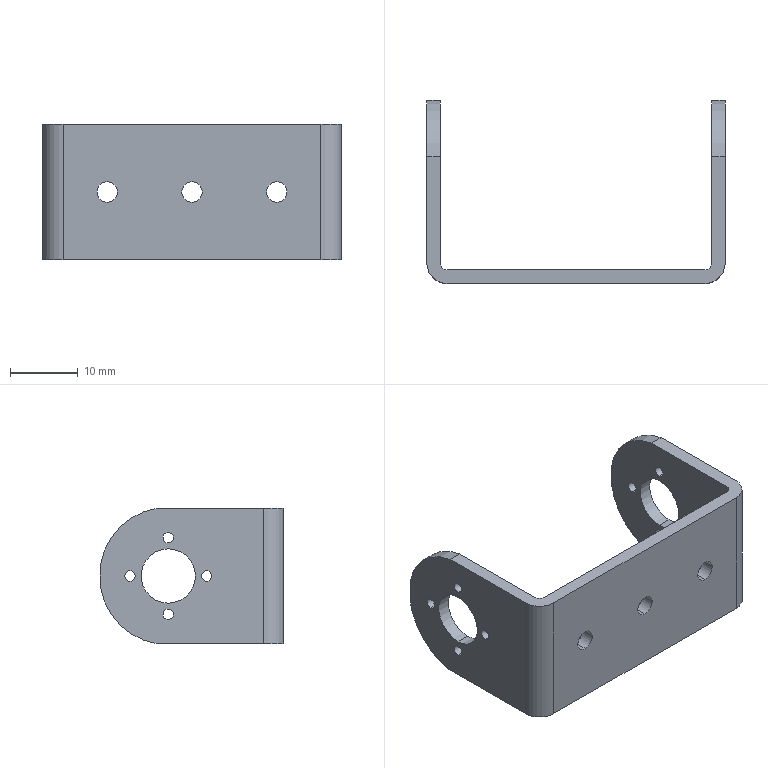Part | SolidWorks | features ICE 2, Extrusion 1 | 1 solid | 44 faces | box 44 x 27 x 20 mm | volume 3261 mm3 | cylinder 34 | plane 10 | commonest cylinder face diameters 1.543 x16 3 x6 8 x4 20.27 x4 2 x2 6 x2
STEP:
#1=CARTESIAN_POINT('',(7.5,-2.,8.5));
#2=VERTEX_POINT('',#1);
#3=CARTESIAN_POINT('',(7.5,-2.,11.5));
#4=VERTEX_POINT('',#3);
#5=CARTESIAN_POINT('',(7.5,-2.,10.));
#6=DIRECTION('',(0.,1.,0.));
#7=DIRECTION('',(0.,0.,1.));
#8=AXIS2_PLACEMENT_3D('',#5,#6,#7);
#9=CIRCLE('',#8,1.5);
#10=EDGE_CURVE('',#2,#4,#9,.T.);
#11=ORIENTED_EDGE('',*,*,#10,.F.);
#12=CARTESIAN_POINT('',(7.5,0.,8.5));
#13=VERTEX_POINT('',#12);
#14=CARTESIAN_POINT('',(7.5,-2.,8.5));
#15=DIRECTION('',(0.,1.,0.));
#16=VECTOR('',#15,1000.);
#17=LINE('',#14,#16);
#18=EDGE_CURVE('',#2,#13,#17,.T.);
#19=ORIENTED_EDGE('',*,*,#18,.T.);
#20=CARTESIAN_POINT('',(7.5,0.,11.5));
#21=VERTEX_POINT('',#20);
#22=CARTESIAN_POINT('',(7.5,0.,10.));
#23=DIRECTION('',(0.,1.,0.));
#24=DIRECTION('',(0.,0.,1.));
#25=AXIS2_PLACEMENT_3D('',#22,#23,#24);
#26=CIRCLE('',#25,1.5);
#27=EDGE_CURVE('',#13,#21,#26,.T.);
#28=ORIENTED_EDGE('',*,*,#27,.T.);
#29=CARTESIAN_POINT('',(7.5,-2.,11.5));
#30=DIRECTION('',(0.,1.,0.));
#31=VECTOR('',#30,1000.);
#32=LINE('',#29,#31);
#33=EDGE_CURVE('',#4,#21,#32,.T.);
#34=ORIENTED_EDGE('',*,*,#33,.F.);
#35=EDGE_LOOP('',(#11,#19,#28,#34));
#36=FACE_OUTER_BOUND('',#35,.T.);
#37=CARTESIAN_POINT('',(7.5,-2.,10.));
#38=DIRECTION('',(0.,1.,0.));
#39=DIRECTION('',(0.,0.,1.));
#40=AXIS2_PLACEMENT_3D('',#37,#38,#39);
#41=CYLINDRICAL_SURFACE('',#40,1.5);
#42=ADVANCED_FACE('',(#36),#41,.F.);
#43=CARTESIAN_POINT('',(20.,-2.,8.5));
#44=VERTEX_POINT('',#43);
#45=CARTESIAN_POINT('',(20.,-2.,11.5));
#46=VERTEX_POINT('',#45);
#47=CARTESIAN_POINT('',(20.,-2.,10.));
#48=DIRECTION('',(0.,1.,0.));
#49=DIRECTION('',(0.,0.,1.));
#50=AXIS2_PLACEMENT_3D('',#47,#48,#49);
#51=CIRCLE('',#50,1.5);
#52=EDGE_CURVE('',#44,#46,#51,.T.);
#53=ORIENTED_EDGE('',*,*,#52,.F.);
#54=CARTESIAN_POINT('',(20.,0.,8.5));
#55=VERTEX_POINT('',#54);
#56=CARTESIAN_POINT('',(20.,-2.,8.5));
#57=DIRECTION('',(0.,1.,0.));
#58=VECTOR('',#57,1000.);
#59=LINE('',#56,#58);
#60=EDGE_CURVE('',#44,#55,#59,.T.);
#61=ORIENTED_EDGE('',*,*,#60,.T.);
#62=CARTESIAN_POINT('',(20.,0.,11.5));
#63=VERTEX_POINT('',#62);
#64=CARTESIAN_POINT('',(20.,0.,10.));
#65=DIRECTION('',(0.,1.,0.));
#66=DIRECTION('',(0.,0.,1.));
#67=AXIS2_PLACEMENT_3D('',#64,#65,#66);
#68=CIRCLE('',#67,1.5);
#69=EDGE_CURVE('',#55,#63,#68,.T.);
#70=ORIENTED_EDGE('',*,*,#69,.T.);
#71=CARTESIAN_POINT('',(20.,-2.,11.5));
#72=DIRECTION('',(0.,1.,0.));
#73=VECTOR('',#72,1000.);
#74=LINE('',#71,#73);
#75=EDGE_CURVE('',#46,#63,#74,.T.);
#76=ORIENTED_EDGE('',*,*,#75,.F.);
#77=EDGE_LOOP('',(#53,#61,#70,#76));
#78=FACE_OUTER_BOUND('',#77,.T.);
#79=CARTESIAN_POINT('',(20.,-2.,10.));
#80=DIRECTION('',(0.,1.,0.));
#81=DIRECTION('',(0.,0.,1.));
#82=AXIS2_PLACEMENT_3D('',#79,#80,#81);
#83=CYLINDRICAL_SURFACE('',#82,1.5);
#84=ADVANCED_FACE('',(#78),#83,.F.);
#85=CARTESIAN_POINT('',(32.5,-2.,8.5));
#86=VERTEX_POINT('',#85);
#87=CARTESIAN_POINT('',(32.5,-2.,11.5));
#88=VERTEX_POINT('',#87);
#89=CARTESIAN_POINT('',(32.5,-2.,10.));
#90=DIRECTION('',(0.,1.,0.));
#91=DIRECTION('',(0.,0.,1.));
#92=AXIS2_PLACEMENT_3D('',#89,#90,#91);
#93=CIRCLE('',#92,1.5);
#94=EDGE_CURVE('',#86,#88,#93,.T.);
#95=ORIENTED_EDGE('',*,*,#94,.F.);
#96=CARTESIAN_POINT('',(32.5,0.,8.5));
#97=VERTEX_POINT('',#96);
#98=CARTESIAN_POINT('',(32.5,-2.,8.5));
#99=DIRECTION('',(0.,1.,0.));
#100=VECTOR('',#99,1000.);
#101=LINE('',#98,#100);
#102=EDGE_CURVE('',#86,#97,#101,.T.);
#103=ORIENTED_EDGE('',*,*,#102,.T.);
#104=CARTESIAN_POINT('',(32.5,0.,11.5));
#105=VERTEX_POINT('',#104);
#106=CARTESIAN_POINT('',(32.5,0.,10.));
#107=DIRECTION('',(0.,1.,0.));
#108=DIRECTION('',(0.,0.,1.));
#109=AXIS2_PLACEMENT_3D('',#106,#107,#108);
#110=CIRCLE('',#109,1.5);
#111=EDGE_CURVE('',#97,#105,#110,.T.);
#112=ORIENTED_EDGE('',*,*,#111,.T.);
#113=CARTESIAN_POINT('',(32.5,-2.,11.5));
#114=DIRECTION('',(0.,1.,0.));
#115=VECTOR('',#114,1000.);
#116=LINE('',#113,#115);
#117=EDGE_CURVE('',#88,#105,#116,.T.);
#118=ORIENTED_EDGE('',*,*,#117,.F.);
#119=EDGE_LOOP('',(#95,#103,#112,#118));
#120=FACE_OUTER_BOUND('',#119,.T.);
#121=CARTESIAN_POINT('',(32.5,-2.,10.));
#122=DIRECTION('',(0.,1.,0.));
#123=DIRECTION('',(0.,0.,1.));
#124=AXIS2_PLACEMENT_3D('',#121,#122,#123);
#125=CYLINDRICAL_SURFACE('',#124,1.5);
#126=ADVANCED_FACE('',(#120),#125,.F.);
#127=CARTESIAN_POINT('',(42.,9.349,9.229));
#128=VERTEX_POINT('',#127);
#129=CARTESIAN_POINT('',(42.,9.349,10.771));
#130=VERTEX_POINT('',#129);
#131=CARTESIAN_POINT('',(42.,9.349,10.));
#132=DIRECTION('',(-1.,0.,0.));
#133=DIRECTION('',(0.,0.,1.));
#134=AXIS2_PLACEMENT_3D('',#131,#132,#133);
#135=CIRCLE('',#134,0.7713);
#136=EDGE_CURVE('',#128,#130,#135,.T.);
#137=ORIENTED_EDGE('',*,*,#136,.F.);
#138=CARTESIAN_POINT('',(40.,9.349,9.229));
#139=VERTEX_POINT('',#138);
#140=CARTESIAN_POINT('',(42.,9.349,9.229));
#141=DIRECTION('',(-1.,0.,0.));
#142=VECTOR('',#141,1000.);
#143=LINE('',#140,#142);
#144=EDGE_CURVE('',#128,#139,#143,.T.);
#145=ORIENTED_EDGE('',*,*,#144,.T.);
#146=CARTESIAN_POINT('',(40.,9.349,10.771));
#147=VERTEX_POINT('',#146);
#148=CARTESIAN_POINT('',(40.,9.349,10.));
#149=DIRECTION('',(1.,0.,0.));
#150=DIRECTION('',(0.,0.,-1.));
#151=AXIS2_PLACEMENT_3D('',#148,#149,#150);
#152=CIRCLE('',#151,0.7713);
#153=EDGE_CURVE('',#147,#139,#152,.T.);
#154=ORIENTED_EDGE('',*,*,#153,.F.);
#155=CARTESIAN_POINT('',(42.,9.349,10.771));
#156=DIRECTION('',(-1.,0.,0.));
#157=VECTOR('',#156,1000.);
#158=LINE('',#155,#157);
#159=EDGE_CURVE('',#130,#147,#158,.T.);
#160=ORIENTED_EDGE('',*,*,#159,.F.);
#161=EDGE_LOOP('',(#137,#145,#154,#160));
#162=FACE_OUTER_BOUND('',#161,.T.);
#163=CARTESIAN_POINT('',(42.,9.349,10.));
#164=DIRECTION('',(-1.,0.,0.));
#165=DIRECTION('',(0.,0.,1.));
#166=AXIS2_PLACEMENT_3D('',#163,#164,#165);
#167=CYLINDRICAL_SURFACE('',#166,0.7713);
#168=ADVANCED_FACE('',(#162),#167,.F.);
#169=CARTESIAN_POINT('',(42.,15.,14.88));
#170=VERTEX_POINT('',#169);
#171=CARTESIAN_POINT('',(42.,15.,16.423));
#172=VERTEX_POINT('',#171);
#173=CARTESIAN_POINT('',(42.,15.,15.651));
#174=DIRECTION('',(-1.,0.,0.));
#175=DIRECTION('',(0.,0.,1.));
#176=AXIS2_PLACEMENT_3D('',#173,#174,#175);
#177=CIRCLE('',#176,0.7713);
#178=EDGE_CURVE('',#170,#172,#177,.T.);
#179=ORIENTED_EDGE('',*,*,#178,.F.);
#180=CARTESIAN_POINT('',(40.,15.,14.88));
#181=VERTEX_POINT('',#180);
#182=CARTESIAN_POINT('',(42.,15.,14.88));
#183=DIRECTION('',(-1.,0.,0.));
#184=VECTOR('',#183,1000.);
#185=LINE('',#182,#184);
#186=EDGE_CURVE('',#170,#181,#185,.T.);
#187=ORIENTED_EDGE('',*,*,#186,.T.);
#188=CARTESIAN_POINT('',(40.,15.,16.423));
#189=VERTEX_POINT('',#188);
#190=CARTESIAN_POINT('',(40.,15.,15.651));
#191=DIRECTION('',(1.,0.,0.));
#192=DIRECTION('',(0.,0.,-1.));
#193=AXIS2_PLACEMENT_3D('',#190,#191,#192);
#194=CIRCLE('',#193,0.7713);
#195=EDGE_CURVE('',#189,#181,#194,.T.);
#196=ORIENTED_EDGE('',*,*,#195,.F.);
#197=CARTESIAN_POINT('',(42.,15.,16.423));
#198=DIRECTION('',(-1.,0.,0.));
#199=VECTOR('',#198,1000.);
#200=LINE('',#197,#199);
#201=EDGE_CURVE('',#172,#189,#200,.T.);
#202=ORIENTED_EDGE('',*,*,#201,.F.);
#203=EDGE_LOOP('',(#179,#187,#196,#202));
#204=FACE_OUTER_BOUND('',#203,.T.);
#205=CARTESIAN_POINT('',(42.,15.,15.651));
#206=DIRECTION('',(-1.,0.,0.));
#207=DIRECTION('',(0.,0.,1.));
#208=AXIS2_PLACEMENT_3D('',#205,#206,#207);
#209=CYLINDRICAL_SURFACE('',#208,0.7713);
#210=ADVANCED_FACE('',(#204),#209,.F.);
#211=CARTESIAN_POINT('',(42.,20.651,9.229));
#212=VERTEX_POINT('',#211);
#213=CARTESIAN_POINT('',(42.,20.651,10.771));
#214=VERTEX_POINT('',#213);
#215=CARTESIAN_POINT('',(42.,20.651,10.));
#216=DIRECTION('',(-1.,0.,0.));
#217=DIRECTION('',(0.,0.,1.));
#218=AXIS2_PLACEMENT_3D('',#215,#216,#217);
#219=CIRCLE('',#218,0.7713);
#220=EDGE_CURVE('',#212,#214,#219,.T.);
#221=ORIENTED_EDGE('',*,*,#220,.F.);
#222=CARTESIAN_POINT('',(40.,20.651,9.229));
#223=VERTEX_POINT('',#222);
#224=CARTESIAN_POINT('',(42.,20.651,9.229));
#225=DIRECTION('',(-1.,0.,0.));
#226=VECTOR('',#225,1000.);
#227=LINE('',#224,#226);
#228=EDGE_CURVE('',#212,#223,#227,.T.);
#229=ORIENTED_EDGE('',*,*,#228,.T.);
#230=CARTESIAN_POINT('',(40.,20.651,10.771));
#231=VERTEX_POINT('',#230);
#232=CARTESIAN_POINT('',(40.,20.651,10.));
#233=DIRECTION('',(1.,0.,0.));
#234=DIRECTION('',(0.,0.,-1.));
#235=AXIS2_PLACEMENT_3D('',#232,#233,#234);
#236=CIRCLE('',#235,0.7713);
#237=EDGE_CURVE('',#231,#223,#236,.T.);
#238=ORIENTED_EDGE('',*,*,#237,.F.);
#239=CARTESIAN_POINT('',(42.,20.651,10.771));
#240=DIRECTION('',(-1.,0.,0.));
#241=VECTOR('',#240,1000.);
#242=LINE('',#239,#241);
#243=EDGE_CURVE('',#214,#231,#242,.T.);
#244=ORIENTED_EDGE('',*,*,#243,.F.);
#245=EDGE_LOOP('',(#221,#229,#238,#244));
#246=FACE_OUTER_BOUND('',#245,.T.);
#247=CARTESIAN_POINT('',(42.,20.651,10.));
#248=DIRECTION('',(-1.,0.,0.));
#249=DIRECTION('',(0.,0.,1.));
#250=AXIS2_PLACEMENT_3D('',#247,#248,#249);
#251=CYLINDRICAL_SURFACE('',#250,0.7713);
#252=ADVANCED_FACE('',(#246),#251,.F.);
#253=CARTESIAN_POINT('',(42.,15.,3.577));
#254=VERTEX_POINT('',#253);
#255=CARTESIAN_POINT('',(42.,15.,5.12));
#256=VERTEX_POINT('',#255);
#257=CARTESIAN_POINT('',(42.,15.,4.349));
#258=DIRECTION('',(-1.,0.,0.));
#259=DIRECTION('',(0.,0.,1.));
#260=AXIS2_PLACEMENT_3D('',#257,#258,#259);
#261=CIRCLE('',#260,0.7713);
#262=EDGE_CURVE('',#254,#256,#261,.T.);
#263=ORIENTED_EDGE('',*,*,#262,.F.);
#264=CARTESIAN_POINT('',(40.,15.,3.577));
#265=VERTEX_POINT('',#264);
#266=CARTESIAN_POINT('',(42.,15.,3.577));
#267=DIRECTION('',(-1.,0.,0.));
#268=VECTOR('',#267,1000.);
#269=LINE('',#266,#268);
#270=EDGE_CURVE('',#254,#265,#269,.T.);
#271=ORIENTED_EDGE('',*,*,#270,.T.);
#272=CARTESIAN_POINT('',(40.,15.,5.12));
#273=VERTEX_POINT('',#272);
#274=CARTESIAN_POINT('',(40.,15.,4.349));
#275=DIRECTION('',(1.,0.,0.));
#276=DIRECTION('',(0.,0.,-1.));
#277=AXIS2_PLACEMENT_3D('',#274,#275,#276);
#278=CIRCLE('',#277,0.7713);
#279=EDGE_CURVE('',#273,#265,#278,.T.);
#280=ORIENTED_EDGE('',*,*,#279,.F.);
#281=CARTESIAN_POINT('',(42.,15.,5.12));
#282=DIRECTION('',(-1.,0.,0.));
#283=VECTOR('',#282,1000.);
#284=LINE('',#281,#283);
#285=EDGE_CURVE('',#256,#273,#284,.T.);
#286=ORIENTED_EDGE('',*,*,#285,.F.);
#287=EDGE_LOOP('',(#263,#271,#280,#286));
#288=FACE_OUTER_BOUND('',#287,.T.);
#289=CARTESIAN_POINT('',(42.,15.,4.349));
#290=DIRECTION('',(-1.,0.,0.));
#291=DIRECTION('',(0.,0.,1.));
#292=AXIS2_PLACEMENT_3D('',#289,#290,#291);
#293=CYLINDRICAL_SURFACE('',#292,0.7713);
#294=ADVANCED_FACE('',(#288),#293,.F.);
#295=CARTESIAN_POINT('',(42.,15.,6.));
#296=VERTEX_POINT('',#295);
#297=CARTESIAN_POINT('',(42.,15.,14.));
#298=VERTEX_POINT('',#297);
#299=CARTESIAN_POINT('',(42.,15.,10.));
#300=DIRECTION('',(-1.,0.,0.));
#301=DIRECTION('',(0.,0.,1.));
#302=AXIS2_PLACEMENT_3D('',#299,#300,#301);
#303=CIRCLE('',#302,4.);
#304=EDGE_CURVE('',#296,#298,#303,.T.);
#305=ORIENTED_EDGE('',*,*,#304,.F.);
#306=CARTESIAN_POINT('',(40.,15.,6.));
#307=VERTEX_POINT('',#306);
#308=CARTESIAN_POINT('',(42.,15.,6.));
#309=DIRECTION('',(-1.,0.,0.));
#310=VECTOR('',#309,1000.);
#311=LINE('',#308,#310);
#312=EDGE_CURVE('',#296,#307,#311,.T.);
#313=ORIENTED_EDGE('',*,*,#312,.T.);
#314=CARTESIAN_POINT('',(40.,15.,14.));
#315=VERTEX_POINT('',#314);
#316=CARTESIAN_POINT('',(40.,15.,10.));
#317=DIRECTION('',(1.,0.,0.));
#318=DIRECTION('',(0.,0.,-1.));
#319=AXIS2_PLACEMENT_3D('',#316,#317,#318);
#320=CIRCLE('',#319,4.);
#321=EDGE_CURVE('',#315,#307,#320,.T.);
#322=ORIENTED_EDGE('',*,*,#321,.F.);
#323=CARTESIAN_POINT('',(42.,15.,14.));
#324=DIRECTION('',(-1.,0.,0.));
#325=VECTOR('',#324,1000.);
#326=LINE('',#323,#325);
#327=EDGE_CURVE('',#298,#315,#326,.T.);
#328=ORIENTED_EDGE('',*,*,#327,.F.);
#329=EDGE_LOOP('',(#305,#313,#322,#328));
#330=FACE_OUTER_BOUND('',#329,.T.);
#331=CARTESIAN_POINT('',(42.,15.,10.));
#332=DIRECTION('',(-1.,0.,0.));
#333=DIRECTION('',(0.,0.,1.));
#334=AXIS2_PLACEMENT_3D('',#331,#332,#333);
#335=CYLINDRICAL_SURFACE('',#334,4.);
#336=ADVANCED_FACE('',(#330),#335,.F.);
#337=CARTESIAN_POINT('',(0.,9.349,9.229));
#338=VERTEX_POINT('',#337);
#339=CARTESIAN_POINT('',(0.,9.349,10.771));
#340=VERTEX_POINT('',#339);
#341=CARTESIAN_POINT('',(0.,9.349,10.));
#342=DIRECTION('',(-1.,0.,0.));
#343=DIRECTION('',(0.,-1.,0.));
#344=AXIS2_PLACEMENT_3D('',#341,#342,#343);
#345=CIRCLE('',#344,0.7713);
#346=EDGE_CURVE('',#338,#340,#345,.T.);
#347=ORIENTED_EDGE('',*,*,#346,.F.);
#348=CARTESIAN_POINT('',(-2.,9.349,9.229));
#349=VERTEX_POINT('',#348);
#350=CARTESIAN_POINT('',(42.,9.349,9.229));
#351=DIRECTION('',(-1.,0.,0.));
#352=VECTOR('',#351,1000.);
#353=LINE('',#350,#352);
#354=EDGE_CURVE('',#338,#349,#353,.T.);
#355=ORIENTED_EDGE('',*,*,#354,.T.);
#356=CARTESIAN_POINT('',(-2.,9.349,10.771));
#357=VERTEX_POINT('',#356);
#358=CARTESIAN_POINT('',(-2.,9.349,10.));
#359=DIRECTION('',(-1.,0.,0.));
#360=DIRECTION('',(0.,0.,1.));
#361=AXIS2_PLACEMENT_3D('',#358,#359,#360);
#362=CIRCLE('',#361,0.7713);
#363=EDGE_CURVE('',#349,#357,#362,.T.);
#364=ORIENTED_EDGE('',*,*,#363,.T.);
#365=CARTESIAN_POINT('',(42.,9.349,10.771));
#366=DIRECTION('',(-1.,0.,0.));
#367=VECTOR('',#366,1000.);
#368=LINE('',#365,#367);
#369=EDGE_CURVE('',#340,#357,#368,.T.);
#370=ORIENTED_EDGE('',*,*,#369,.F.);
#371=EDGE_LOOP('',(#347,#355,#364,#370));
#372=FACE_OUTER_BOUND('',#371,.T.);
#373=CARTESIAN_POINT('',(42.,9.349,10.));
#374=DIRECTION('',(-1.,0.,0.));
#375=DIRECTION('',(0.,0.,1.));
#376=AXIS2_PLACEMENT_3D('',#373,#374,#375);
#377=CYLINDRICAL_SURFACE('',#376,0.7713);
#378=ADVANCED_FACE('',(#372),#377,.F.);
#379=CARTESIAN_POINT('',(0.,15.,14.88));
#380=VERTEX_POINT('',#379);
#381=CARTESIAN_POINT('',(0.,15.,16.423));
#382=VERTEX_POINT('',#381);
#383=CARTESIAN_POINT('',(0.,15.,15.651));
#384=DIRECTION('',(-1.,0.,0.));
#385=DIRECTION('',(0.,-1.,0.));
#386=AXIS2_PLACEMENT_3D('',#383,#384,#385);
#387=CIRCLE('',#386,0.7713);
#388=EDGE_CURVE('',#380,#382,#387,.T.);
#389=ORIENTED_EDGE('',*,*,#388,.F.);
#390=CARTESIAN_POINT('',(-2.,15.,14.88));
#391=VERTEX_POINT('',#390);
#392=CARTESIAN_POINT('',(42.,15.,14.88));
#393=DIRECTION('',(-1.,0.,0.));
#394=VECTOR('',#393,1000.);
#395=LINE('',#392,#394);
#396=EDGE_CURVE('',#380,#391,#395,.T.);
#397=ORIENTED_EDGE('',*,*,#396,.T.);
#398=CARTESIAN_POINT('',(-2.,15.,16.423));
#399=VERTEX_POINT('',#398);
#400=CARTESIAN_POINT('',(-2.,15.,15.651));
#401=DIRECTION('',(-1.,0.,0.));
#402=DIRECTION('',(0.,0.,1.));
#403=AXIS2_PLACEMENT_3D('',#400,#401,#402);
#404=CIRCLE('',#403,0.7713);
#405=EDGE_CURVE('',#391,#399,#404,.T.);
#406=ORIENTED_EDGE('',*,*,#405,.T.);
#407=CARTESIAN_POINT('',(42.,15.,16.423));
#408=DIRECTION('',(-1.,0.,0.));
#409=VECTOR('',#408,1000.);
#410=LINE('',#407,#409);
#411=EDGE_CURVE('',#382,#399,#410,.T.);
#412=ORIENTED_EDGE('',*,*,#411,.F.);
#413=EDGE_LOOP('',(#389,#397,#406,#412));
#414=FACE_OUTER_BOUND('',#413,.T.);
#415=CARTESIAN_POINT('',(42.,15.,15.651));
#416=DIRECTION('',(-1.,0.,0.));
#417=DIRECTION('',(0.,0.,1.));
#418=AXIS2_PLACEMENT_3D('',#415,#416,#417);
#419=CYLINDRICAL_SURFACE('',#418,0.7713);
#420=ADVANCED_FACE('',(#414),#419,.F.);
#421=CARTESIAN_POINT('',(0.,20.651,9.229));
#422=VERTEX_POINT('',#421);
#423=CARTESIAN_POINT('',(0.,20.651,10.771));
#424=VERTEX_POINT('',#423);
#425=CARTESIAN_POINT('',(0.,20.651,10.));
#426=DIRECTION('',(-1.,0.,0.));
#427=DIRECTION('',(0.,-1.,0.));
#428=AXIS2_PLACEMENT_3D('',#425,#426,#427);
#429=CIRCLE('',#428,0.7713);
#430=EDGE_CURVE('',#422,#424,#429,.T.);
#431=ORIENTED_EDGE('',*,*,#430,.F.);
#432=CARTESIAN_POINT('',(-2.,20.651,9.229));
#433=VERTEX_POINT('',#432);
#434=CARTESIAN_POINT('',(42.,20.651,9.229));
#435=DIRECTION('',(-1.,0.,0.));
#436=VECTOR('',#435,1000.);
#437=LINE('',#434,#436);
#438=EDGE_CURVE('',#422,#433,#437,.T.);
#439=ORIENTED_EDGE('',*,*,#438,.T.);
#440=CARTESIAN_POINT('',(-2.,20.651,10.771));
#441=VERTEX_POINT('',#440);
#442=CARTESIAN_POINT('',(-2.,20.651,10.));
#443=DIRECTION('',(-1.,0.,0.));
#444=DIRECTION('',(0.,0.,1.));
#445=AXIS2_PLACEMENT_3D('',#442,#443,#444);
#446=CIRCLE('',#445,0.7713);
#447=EDGE_CURVE('',#433,#441,#446,.T.);
#448=ORIENTED_EDGE('',*,*,#447,.T.);
#449=CARTESIAN_POINT('',(42.,20.651,10.771));
#450=DIRECTION('',(-1.,0.,0.));
#451=VECTOR('',#450,1000.);
#452=LINE('',#449,#451);
#453=EDGE_CURVE('',#424,#441,#452,.T.);
#454=ORIENTED_EDGE('',*,*,#453,.F.);
#455=EDGE_LOOP('',(#431,#439,#448,#454));
#456=FACE_OUTER_BOUND('',#455,.T.);
#457=CARTESIAN_POINT('',(42.,20.651,10.));
#458=DIRECTION('',(-1.,0.,0.));
#459=DIRECTION('',(0.,0.,1.));
#460=AXIS2_PLACEMENT_3D('',#457,#458,#459);
#461=CYLINDRICAL_SURFACE('',#460,0.7713);
#462=ADVANCED_FACE('',(#456),#461,.F.);
#463=CARTESIAN_POINT('',(0.,15.,3.577));
#464=VERTEX_POINT('',#463);
#465=CARTESIAN_POINT('',(0.,15.,5.12));
#466=VERTEX_POINT('',#465);
#467=CARTESIAN_POINT('',(0.,15.,4.349));
#468=DIRECTION('',(-1.,0.,0.));
#469=DIRECTION('',(0.,-1.,0.));
#470=AXIS2_PLACEMENT_3D('',#467,#468,#469);
#471=CIRCLE('',#470,0.7713);
#472=EDGE_CURVE('',#464,#466,#471,.T.);
#473=ORIENTED_EDGE('',*,*,#472,.F.);
#474=CARTESIAN_POINT('',(-2.,15.,3.577));
#475=VERTEX_POINT('',#474);
#476=CARTESIAN_POINT('',(42.,15.,3.577));
#477=DIRECTION('',(-1.,0.,0.));
#478=VECTOR('',#477,1000.);
#479=LINE('',#476,#478);
#480=EDGE_CURVE('',#464,#475,#479,.T.);
#481=ORIENTED_EDGE('',*,*,#480,.T.);
#482=CARTESIAN_POINT('',(-2.,15.,5.12));
#483=VERTEX_POINT('',#482);
#484=CARTESIAN_POINT('',(-2.,15.,4.349));
#485=DIRECTION('',(-1.,0.,0.));
#486=DIRECTION('',(0.,0.,1.));
#487=AXIS2_PLACEMENT_3D('',#484,#485,#486);
#488=CIRCLE('',#487,0.7713);
#489=EDGE_CURVE('',#475,#483,#488,.T.);
#490=ORIENTED_EDGE('',*,*,#489,.T.);
#491=CARTESIAN_POINT('',(42.,15.,5.12));
#492=DIRECTION('',(-1.,0.,0.));
#493=VECTOR('',#492,1000.);
#494=LINE('',#491,#493);
#495=EDGE_CURVE('',#466,#483,#494,.T.);
#496=ORIENTED_EDGE('',*,*,#495,.F.);
#497=EDGE_LOOP('',(#473,#481,#490,#496));
#498=FACE_OUTER_BOUND('',#497,.T.);
#499=CARTESIAN_POINT('',(42.,15.,4.349));
#500=DIRECTION('',(-1.,0.,0.));
#501=DIRECTION('',(0.,0.,1.));
#502=AXIS2_PLACEMENT_3D('',#499,#500,#501);
#503=CYLINDRICAL_SURFACE('',#502,0.7713);
#504=ADVANCED_FACE('',(#498),#503,.F.);
#505=CARTESIAN_POINT('',(0.,15.,6.));
#506=VERTEX_POINT('',#505);
#507=CARTESIAN_POINT('',(0.,15.,14.));
#508=VERTEX_POINT('',#507);
#509=CARTESIAN_POINT('',(0.,15.,10.));
#510=DIRECTION('',(-1.,0.,0.));
#511=DIRECTION('',(0.,-1.,0.));
#512=AXIS2_PLACEMENT_3D('',#509,#510,#511);
#513=CIRCLE('',#512,4.);
#514=EDGE_CURVE('',#506,#508,#513,.T.);
#515=ORIENTED_EDGE('',*,*,#514,.F.);
#516=CARTESIAN_POINT('',(-2.,15.,6.));
#517=VERTEX_POINT('',#516);
#518=CARTESIAN_POINT('',(42.,15.,6.));
#519=DIRECTION('',(-1.,0.,0.));
#520=VECTOR('',#519,1000.);
#521=LINE('',#518,#520);
#522=EDGE_CURVE('',#506,#517,#521,.T.);
#523=ORIENTED_EDGE('',*,*,#522,.T.);
#524=CARTESIAN_POINT('',(-2.,15.,14.));
#525=VERTEX_POINT('',#524);
#526=CARTESIAN_POINT('',(-2.,15.,10.));
#527=DIRECTION('',(-1.,0.,0.));
#528=DIRECTION('',(0.,0.,1.));
#529=AXIS2_PLACEMENT_3D('',#526,#527,#528);
#530=CIRCLE('',#529,4.);
#531=EDGE_CURVE('',#517,#525,#530,.T.);
#532=ORIENTED_EDGE('',*,*,#531,.T.);
#533=CARTESIAN_POINT('',(42.,15.,14.));
#534=DIRECTION('',(-1.,0.,0.));
#535=VECTOR('',#534,1000.);
#536=LINE('',#533,#535);
#537=EDGE_CURVE('',#508,#525,#536,.T.);
#538=ORIENTED_EDGE('',*,*,#537,.F.);
#539=EDGE_LOOP('',(#515,#523,#532,#538));
#540=FACE_OUTER_BOUND('',#539,.T.);
#541=CARTESIAN_POINT('',(42.,15.,10.));
#542=DIRECTION('',(-1.,0.,0.));
#543=DIRECTION('',(0.,0.,1.));
#544=AXIS2_PLACEMENT_3D('',#541,#542,#543);
#545=CYLINDRICAL_SURFACE('',#544,4.);
#546=ADVANCED_FACE('',(#540),#545,.F.);
#547=CARTESIAN_POINT('',(-2.,25.,11.647));
#548=VERTEX_POINT('',#547);
#549=CARTESIAN_POINT('',(-2.,25.,8.353));
#550=VERTEX_POINT('',#549);
#551=CARTESIAN_POINT('',(-2.,25.,20.));
#552=DIRECTION('',(0.,0.,-1.));
#553=VECTOR('',#552,1000.);
#554=LINE('',#551,#553);
#555=EDGE_CURVE('',#548,#550,#554,.T.);
#556=ORIENTED_EDGE('',*,*,#555,.F.);
#557=CARTESIAN_POINT('',(0.,25.,11.647));
#558=VERTEX_POINT('',#557);
#559=CARTESIAN_POINT('',(42.,25.,11.647));
#560=DIRECTION('',(1.,0.,0.));
#561=VECTOR('',#560,1000.);
#562=LINE('',#559,#561);
#563=EDGE_CURVE('',#548,#558,#562,.T.);
#564=ORIENTED_EDGE('',*,*,#563,.T.);
#565=CARTESIAN_POINT('',(0.,25.,8.353));
#566=VERTEX_POINT('',#565);
#567=CARTESIAN_POINT('',(0.,25.,20.));
#568=DIRECTION('',(0.,0.,-1.));
#569=VECTOR('',#568,1000.);
#570=LINE('',#567,#569);
#571=EDGE_CURVE('',#558,#566,#570,.T.);
#572=ORIENTED_EDGE('',*,*,#571,.T.);
#573=CARTESIAN_POINT('',(42.,25.,8.353));
#574=DIRECTION('',(-1.,0.,0.));
#575=VECTOR('',#574,1000.);
#576=LINE('',#573,#575);
#577=EDGE_CURVE('',#566,#550,#576,.T.);
#578=ORIENTED_EDGE('',*,*,#577,.T.);
#579=EDGE_LOOP('',(#556,#564,#572,#578));
#580=FACE_OUTER_BOUND('',#579,.T.);
#581=CARTESIAN_POINT('',(-2.,25.,20.));
#582=DIRECTION('',(0.,-1.,0.));
#583=DIRECTION('',(0.,0.,-1.));
#584=AXIS2_PLACEMENT_3D('',#581,#582,#583);
#585=PLANE('',#584);
#586=ADVANCED_FACE('',(#580),#585,.F.);
#587=CARTESIAN_POINT('',(-2.,9.349,10.));
#588=DIRECTION('',(-1.,0.,0.));
#589=DIRECTION('',(0.,0.,1.));
#590=AXIS2_PLACEMENT_3D('',#587,#588,#589);
#591=CIRCLE('',#590,0.7713);
#592=EDGE_CURVE('',#357,#349,#591,.T.);
#593=ORIENTED_EDGE('',*,*,#592,.F.);
#594=ORIENTED_EDGE('',*,*,#363,.F.);
#595=EDGE_LOOP('',(#593,#594));
#596=FACE_BOUND('',#595,.T.);
#597=CARTESIAN_POINT('',(-2.,15.,15.651));
#598=DIRECTION('',(-1.,0.,0.));
#599=DIRECTION('',(0.,0.,1.));
#600=AXIS2_PLACEMENT_3D('',#597,#598,#599);
#601=CIRCLE('',#600,0.7713);
#602=EDGE_CURVE('',#399,#391,#601,.T.);
#603=ORIENTED_EDGE('',*,*,#602,.F.);
#604=ORIENTED_EDGE('',*,*,#405,.F.);
#605=EDGE_LOOP('',(#603,#604));
#606=FACE_BOUND('',#605,.T.);
#607=CARTESIAN_POINT('',(-2.,20.651,10.));
#608=DIRECTION('',(-1.,0.,0.));
#609=DIRECTION('',(0.,0.,1.));
#610=AXIS2_PLACEMENT_3D('',#607,#608,#609);
#611=CIRCLE('',#610,0.7713);
#612=EDGE_CURVE('',#441,#433,#611,.T.);
#613=ORIENTED_EDGE('',*,*,#612,.F.);
#614=ORIENTED_EDGE('',*,*,#447,.F.);
#615=EDGE_LOOP('',(#613,#614));
#616=FACE_BOUND('',#615,.T.);
#617=CARTESIAN_POINT('',(-2.,15.,4.349));
#618=DIRECTION('',(-1.,0.,0.));
#619=DIRECTION('',(0.,0.,1.));
#620=AXIS2_PLACEMENT_3D('',#617,#618,#619);
#621=CIRCLE('',#620,0.7713);
#622=EDGE_CURVE('',#483,#475,#621,.T.);
#623=ORIENTED_EDGE('',*,*,#622,.F.);
#624=ORIENTED_EDGE('',*,*,#489,.F.);
#625=EDGE_LOOP('',(#623,#624));
#626=FACE_BOUND('',#625,.T.);
#627=CARTESIAN_POINT('',(-2.,15.,10.));
#628=DIRECTION('',(-1.,0.,0.));
#629=DIRECTION('',(0.,0.,1.));
#630=AXIS2_PLACEMENT_3D('',#627,#628,#629);
#631=CIRCLE('',#630,4.);
#632=EDGE_CURVE('',#525,#517,#631,.T.);
#633=ORIENTED_EDGE('',*,*,#632,.F.);
#634=ORIENTED_EDGE('',*,*,#531,.F.);
#635=EDGE_LOOP('',(#633,#634));
#636=FACE_BOUND('',#635,.T.);
#637=CARTESIAN_POINT('',(-2.,16.647,20.));
#638=VERTEX_POINT('',#637);
#639=CARTESIAN_POINT('',(-2.,1.,20.));
#640=VERTEX_POINT('',#639);
#641=CARTESIAN_POINT('',(-2.,25.,20.));
#642=DIRECTION('',(0.,-1.,0.));
#643=VECTOR('',#642,1000.);
#644=LINE('',#641,#643);
#645=EDGE_CURVE('',#638,#640,#644,.T.);
#646=ORIENTED_EDGE('',*,*,#645,.F.);
#647=CARTESIAN_POINT('',(-2.,15.,10.));
#648=DIRECTION('',(1.,0.,0.));
#649=DIRECTION('',(0.,0.,1.));
#650=AXIS2_PLACEMENT_3D('',#647,#648,#649);
#651=CIRCLE('',#650,10.135);
#652=EDGE_CURVE('',#548,#638,#651,.T.);
#653=ORIENTED_EDGE('',*,*,#652,.F.);
#654=ORIENTED_EDGE('',*,*,#555,.T.);
#655=CARTESIAN_POINT('',(-2.,16.647,0.));
#656=VERTEX_POINT('',#655);
#657=CARTESIAN_POINT('',(-2.,15.,10.));
#658=DIRECTION('',(1.,0.,0.));
#659=DIRECTION('',(0.,0.,1.));
#660=AXIS2_PLACEMENT_3D('',#657,#658,#659);
#661=CIRCLE('',#660,10.135);
#662=EDGE_CURVE('',#656,#550,#661,.T.);
#663=ORIENTED_EDGE('',*,*,#662,.F.);
#664=CARTESIAN_POINT('',(-2.,1.,0.));
#665=VERTEX_POINT('',#664);
#666=CARTESIAN_POINT('',(-2.,25.,0.));
#667=DIRECTION('',(0.,-1.,0.));
#668=VECTOR('',#667,1000.);
#669=LINE('',#666,#668);
#670=EDGE_CURVE('',#656,#665,#669,.T.);
#671=ORIENTED_EDGE('',*,*,#670,.T.);
#672=CARTESIAN_POINT('',(-2.,1.,20.));
#673=DIRECTION('',(0.,0.,-1.));
#674=VECTOR('',#673,1000.);
#675=LINE('',#672,#674);
#676=EDGE_CURVE('',#640,#665,#675,.T.);
#677=ORIENTED_EDGE('',*,*,#676,.F.);
#678=EDGE_LOOP('',(#646,#653,#654,#663,#671,#677));
#679=FACE_OUTER_BOUND('',#678,.T.);
#680=CARTESIAN_POINT('',(-2.,25.,20.));
#681=DIRECTION('',(1.,0.,0.));
#682=DIRECTION('',(0.,0.,-1.));
#683=AXIS2_PLACEMENT_3D('',#680,#681,#682);
#684=PLANE('',#683);
#685=ADVANCED_FACE('',(#596,#606,#616,#626,#636,#679),#684,.F.);
#686=CARTESIAN_POINT('',(1.,-2.,0.));
#687=VERTEX_POINT('',#686);
#688=CARTESIAN_POINT('',(1.,1.,0.));
#689=DIRECTION('',(0.,0.,1.));
#690=DIRECTION('',(1.,0.,0.));
#691=AXIS2_PLACEMENT_3D('',#688,#689,#690);
#692=CIRCLE('',#691,3.);
#693=EDGE_CURVE('',#665,#687,#692,.T.);
#694=ORIENTED_EDGE('',*,*,#693,.T.);
#695=CARTESIAN_POINT('',(1.,-2.,20.));
#696=VERTEX_POINT('',#695);
#697=CARTESIAN_POINT('',(1.,-2.,20.));
#698=DIRECTION('',(0.,0.,-1.));
#699=VECTOR('',#698,1000.);
#700=LINE('',#697,#699);
#701=EDGE_CURVE('',#696,#687,#700,.T.);
#702=ORIENTED_EDGE('',*,*,#701,.F.);
#703=CARTESIAN_POINT('',(1.,1.,20.));
#704=DIRECTION('',(0.,0.,1.));
#705=DIRECTION('',(1.,0.,0.));
#706=AXIS2_PLACEMENT_3D('',#703,#704,#705);
#707=CIRCLE('',#706,3.);
#708=EDGE_CURVE('',#640,#696,#707,.T.);
#709=ORIENTED_EDGE('',*,*,#708,.F.);
#710=ORIENTED_EDGE('',*,*,#676,.T.);
#711=EDGE_LOOP('',(#694,#702,#709,#710));
#712=FACE_OUTER_BOUND('',#711,.T.);
#713=CARTESIAN_POINT('',(1.,1.,20.));
#714=DIRECTION('',(0.,0.,-1.));
#715=DIRECTION('',(-1.,0.,0.));
#716=AXIS2_PLACEMENT_3D('',#713,#714,#715);
#717=CYLINDRICAL_SURFACE('',#716,3.);
#718=ADVANCED_FACE('',(#712),#717,.T.);
#719=CARTESIAN_POINT('',(7.5,-2.,10.));
#720=DIRECTION('',(0.,1.,0.));
#721=DIRECTION('',(0.,0.,1.));
#722=AXIS2_PLACEMENT_3D('',#719,#720,#721);
#723=CIRCLE('',#722,1.5);
#724=EDGE_CURVE('',#4,#2,#723,.T.);
#725=ORIENTED_EDGE('',*,*,#724,.T.);
#726=ORIENTED_EDGE('',*,*,#10,.T.);
#727=EDGE_LOOP('',(#725,#726));
#728=FACE_BOUND('',#727,.T.);
#729=CARTESIAN_POINT('',(20.,-2.,10.));
#730=DIRECTION('',(0.,1.,0.));
#731=DIRECTION('',(0.,0.,1.));
#732=AXIS2_PLACEMENT_3D('',#729,#730,#731);
#733=CIRCLE('',#732,1.5);
#734=EDGE_CURVE('',#46,#44,#733,.T.);
#735=ORIENTED_EDGE('',*,*,#734,.T.);
#736=ORIENTED_EDGE('',*,*,#52,.T.);
#737=EDGE_LOOP('',(#735,#736));
#738=FACE_BOUND('',#737,.T.);
#739=CARTESIAN_POINT('',(32.5,-2.,10.));
#740=DIRECTION('',(0.,1.,0.));
#741=DIRECTION('',(0.,0.,1.));
#742=AXIS2_PLACEMENT_3D('',#739,#740,#741);
#743=CIRCLE('',#742,1.5);
#744=EDGE_CURVE('',#88,#86,#743,.T.);
#745=ORIENTED_EDGE('',*,*,#744,.T.);
#746=ORIENTED_EDGE('',*,*,#94,.T.);
#747=EDGE_LOOP('',(#745,#746));
#748=FACE_BOUND('',#747,.T.);
#749=CARTESIAN_POINT('',(39.,-2.,0.));
#750=VERTEX_POINT('',#749);
#751=CARTESIAN_POINT('',(1.,-2.,0.));
#752=DIRECTION('',(1.,0.,0.));
#753=VECTOR('',#752,1000.);
#754=LINE('',#751,#753);
#755=EDGE_CURVE('',#687,#750,#754,.T.);
#756=ORIENTED_EDGE('',*,*,#755,.T.);
#757=CARTESIAN_POINT('',(39.,-2.,20.));
#758=VERTEX_POINT('',#757);
#759=CARTESIAN_POINT('',(39.,-2.,20.));
#760=DIRECTION('',(0.,0.,-1.));
#761=VECTOR('',#760,1000.);
#762=LINE('',#759,#761);
#763=EDGE_CURVE('',#758,#750,#762,.T.);
#764=ORIENTED_EDGE('',*,*,#763,.F.);
#765=CARTESIAN_POINT('',(1.,-2.,20.));
#766=DIRECTION('',(1.,0.,0.));
#767=VECTOR('',#766,1000.);
#768=LINE('',#765,#767);
#769=EDGE_CURVE('',#696,#758,#768,.T.);
#770=ORIENTED_EDGE('',*,*,#769,.F.);
#771=ORIENTED_EDGE('',*,*,#701,.T.);
#772=EDGE_LOOP('',(#756,#764,#770,#771));
#773=FACE_OUTER_BOUND('',#772,.T.);
#774=CARTESIAN_POINT('',(1.,-2.,20.));
#775=DIRECTION('',(0.,1.,0.));
#776=DIRECTION('',(0.,0.,1.));
#777=AXIS2_PLACEMENT_3D('',#774,#775,#776);
#778=PLANE('',#777);
#779=ADVANCED_FACE('',(#728,#738,#748,#773),#778,.F.);
#780=CARTESIAN_POINT('',(42.,1.,0.));
#781=VERTEX_POINT('',#780);
#782=CARTESIAN_POINT('',(39.,1.,0.));
#783=DIRECTION('',(0.,0.,1.));
#784=DIRECTION('',(1.,0.,0.));
#785=AXIS2_PLACEMENT_3D('',#782,#783,#784);
#786=CIRCLE('',#785,3.);
#787=EDGE_CURVE('',#750,#781,#786,.T.);
#788=ORIENTED_EDGE('',*,*,#787,.T.);
#789=CARTESIAN_POINT('',(42.,1.,20.));
#790=VERTEX_POINT('',#789);
#791=CARTESIAN_POINT('',(42.,1.,20.));
#792=DIRECTION('',(0.,0.,-1.));
#793=VECTOR('',#792,1000.);
#794=LINE('',#791,#793);
#795=EDGE_CURVE('',#790,#781,#794,.T.);
#796=ORIENTED_EDGE('',*,*,#795,.F.);
#797=CARTESIAN_POINT('',(39.,1.,20.));
#798=DIRECTION('',(0.,0.,1.));
#799=DIRECTION('',(1.,0.,0.));
#800=AXIS2_PLACEMENT_3D('',#797,#798,#799);
#801=CIRCLE('',#800,3.);
#802=EDGE_CURVE('',#758,#790,#801,.T.);
#803=ORIENTED_EDGE('',*,*,#802,.F.);
#804=ORIENTED_EDGE('',*,*,#763,.T.);
#805=EDGE_LOOP('',(#788,#796,#803,#804));
#806=FACE_OUTER_BOUND('',#805,.T.);
#807=CARTESIAN_POINT('',(39.,1.,20.));
#808=DIRECTION('',(0.,0.,-1.));
#809=DIRECTION('',(-1.,0.,0.));
#810=AXIS2_PLACEMENT_3D('',#807,#808,#809);
#811=CYLINDRICAL_SURFACE('',#810,3.);
#812=ADVANCED_FACE('',(#806),#811,.T.);
#813=CARTESIAN_POINT('',(42.,9.349,10.));
#814=DIRECTION('',(-1.,0.,0.));
#815=DIRECTION('',(0.,0.,1.));
#816=AXIS2_PLACEMENT_3D('',#813,#814,#815);
#817=CIRCLE('',#816,0.7713);
#818=EDGE_CURVE('',#130,#128,#817,.T.);
#819=ORIENTED_EDGE('',*,*,#818,.T.);
#820=ORIENTED_EDGE('',*,*,#136,.T.);
#821=EDGE_LOOP('',(#819,#820));
#822=FACE_BOUND('',#821,.T.);
#823=CARTESIAN_POINT('',(42.,15.,15.651));
#824=DIRECTION('',(-1.,0.,0.));
#825=DIRECTION('',(0.,0.,1.));
#826=AXIS2_PLACEMENT_3D('',#823,#824,#825);
#827=CIRCLE('',#826,0.7713);
#828=EDGE_CURVE('',#172,#170,#827,.T.);
#829=ORIENTED_EDGE('',*,*,#828,.T.);
#830=ORIENTED_EDGE('',*,*,#178,.T.);
#831=EDGE_LOOP('',(#829,#830));
#832=FACE_BOUND('',#831,.T.);
#833=CARTESIAN_POINT('',(42.,20.651,10.));
#834=DIRECTION('',(-1.,0.,0.));
#835=DIRECTION('',(0.,0.,1.));
#836=AXIS2_PLACEMENT_3D('',#833,#834,#835);
#837=CIRCLE('',#836,0.7713);
#838=EDGE_CURVE('',#214,#212,#837,.T.);
#839=ORIENTED_EDGE('',*,*,#838,.T.);
#840=ORIENTED_EDGE('',*,*,#220,.T.);
#841=EDGE_LOOP('',(#839,#840));
#842=FACE_BOUND('',#841,.T.);
#843=CARTESIAN_POINT('',(42.,15.,4.349));
#844=DIRECTION('',(-1.,0.,0.));
#845=DIRECTION('',(0.,0.,1.));
#846=AXIS2_PLACEMENT_3D('',#843,#844,#845);
#847=CIRCLE('',#846,0.7713);
#848=EDGE_CURVE('',#256,#254,#847,.T.);
#849=ORIENTED_EDGE('',*,*,#848,.T.);
#850=ORIENTED_EDGE('',*,*,#262,.T.);
#851=EDGE_LOOP('',(#849,#850));
#852=FACE_BOUND('',#851,.T.);
#853=CARTESIAN_POINT('',(42.,15.,10.));
#854=DIRECTION('',(-1.,0.,0.));
#855=DIRECTION('',(0.,0.,1.));
#856=AXIS2_PLACEMENT_3D('',#853,#854,#855);
#857=CIRCLE('',#856,4.);
#858=EDGE_CURVE('',#298,#296,#857,.T.);
#859=ORIENTED_EDGE('',*,*,#858,.T.);
#860=ORIENTED_EDGE('',*,*,#304,.T.);
#861=EDGE_LOOP('',(#859,#860));
#862=FACE_BOUND('',#861,.T.);
#863=CARTESIAN_POINT('',(42.,16.647,0.));
#864=VERTEX_POINT('',#863);
#865=CARTESIAN_POINT('',(42.,1.,0.));
#866=DIRECTION('',(0.,1.,0.));
#867=VECTOR('',#866,1000.);
#868=LINE('',#865,#867);
#869=EDGE_CURVE('',#781,#864,#868,.T.);
#870=ORIENTED_EDGE('',*,*,#869,.T.);
#871=CARTESIAN_POINT('',(42.,25.,8.353));
#872=VERTEX_POINT('',#871);
#873=CARTESIAN_POINT('',(42.,15.,10.));
#874=DIRECTION('',(1.,0.,0.));
#875=DIRECTION('',(0.,0.,1.));
#876=AXIS2_PLACEMENT_3D('',#873,#874,#875);
#877=CIRCLE('',#876,10.135);
#878=EDGE_CURVE('',#864,#872,#877,.T.);
#879=ORIENTED_EDGE('',*,*,#878,.T.);
#880=CARTESIAN_POINT('',(42.,25.,11.647));
#881=VERTEX_POINT('',#880);
#882=CARTESIAN_POINT('',(42.,25.,20.));
#883=DIRECTION('',(0.,0.,-1.));
#884=VECTOR('',#883,1000.);
#885=LINE('',#882,#884);
#886=EDGE_CURVE('',#881,#872,#885,.T.);
#887=ORIENTED_EDGE('',*,*,#886,.F.);
#888=CARTESIAN_POINT('',(42.,16.647,20.));
#889=VERTEX_POINT('',#888);
#890=CARTESIAN_POINT('',(42.,15.,10.));
#891=DIRECTION('',(1.,0.,0.));
#892=DIRECTION('',(0.,0.,1.));
#893=AXIS2_PLACEMENT_3D('',#890,#891,#892);
#894=CIRCLE('',#893,10.135);
#895=EDGE_CURVE('',#881,#889,#894,.T.);
#896=ORIENTED_EDGE('',*,*,#895,.T.);
#897=CARTESIAN_POINT('',(42.,1.,20.));
#898=DIRECTION('',(0.,1.,0.));
#899=VECTOR('',#898,1000.);
#900=LINE('',#897,#899);
#901=EDGE_CURVE('',#790,#889,#900,.T.);
#902=ORIENTED_EDGE('',*,*,#901,.F.);
#903=ORIENTED_EDGE('',*,*,#795,.T.);
#904=EDGE_LOOP('',(#870,#879,#887,#896,#902,#903));
#905=FACE_OUTER_BOUND('',#904,.T.);
#906=CARTESIAN_POINT('',(42.,1.,20.));
#907=DIRECTION('',(-1.,0.,0.));
#908=DIRECTION('',(0.,0.,1.));
#909=AXIS2_PLACEMENT_3D('',#906,#907,#908);
#910=PLANE('',#909);
#911=ADVANCED_FACE('',(#822,#832,#842,#852,#862,#905),#910,.F.);
#912=CARTESIAN_POINT('',(40.,25.,11.647));
#913=VERTEX_POINT('',#912);
#914=CARTESIAN_POINT('',(40.,25.,8.353));
#915=VERTEX_POINT('',#914);
#916=CARTESIAN_POINT('',(40.,25.,20.));
#917=DIRECTION('',(0.,0.,-1.));
#918=VECTOR('',#917,1000.);
#919=LINE('',#916,#918);
#920=EDGE_CURVE('',#913,#915,#919,.T.);
#921=ORIENTED_EDGE('',*,*,#920,.F.);
#922=CARTESIAN_POINT('',(42.,25.,11.647));
#923=DIRECTION('',(1.,0.,0.));
#924=VECTOR('',#923,1000.);
#925=LINE('',#922,#924);
#926=EDGE_CURVE('',#913,#881,#925,.T.);
#927=ORIENTED_EDGE('',*,*,#926,.T.);
#928=ORIENTED_EDGE('',*,*,#886,.T.);
#929=CARTESIAN_POINT('',(42.,25.,8.353));
#930=DIRECTION('',(-1.,0.,0.));
#931=VECTOR('',#930,1000.);
#932=LINE('',#929,#931);
#933=EDGE_CURVE('',#872,#915,#932,.T.);
#934=ORIENTED_EDGE('',*,*,#933,.T.);
#935=EDGE_LOOP('',(#921,#927,#928,#934));
#936=FACE_OUTER_BOUND('',#935,.T.);
#937=CARTESIAN_POINT('',(40.,25.,20.));
#938=DIRECTION('',(0.,-1.,0.));
#939=DIRECTION('',(0.,0.,-1.));
#940=AXIS2_PLACEMENT_3D('',#937,#938,#939);
#941=PLANE('',#940);
#942=ADVANCED_FACE('',(#936),#941,.F.);
#943=ORIENTED_EDGE('',*,*,#153,.T.);
#944=CARTESIAN_POINT('',(40.,9.349,10.));
#945=DIRECTION('',(1.,0.,0.));
#946=DIRECTION('',(0.,0.,-1.));
#947=AXIS2_PLACEMENT_3D('',#944,#945,#946);
#948=CIRCLE('',#947,0.7713);
#949=EDGE_CURVE('',#139,#147,#948,.T.);
#950=ORIENTED_EDGE('',*,*,#949,.T.);
#951=EDGE_LOOP('',(#943,#950));
#952=FACE_BOUND('',#951,.T.);
#953=ORIENTED_EDGE('',*,*,#195,.T.);
#954=CARTESIAN_POINT('',(40.,15.,15.651));
#955=DIRECTION('',(1.,0.,0.));
#956=DIRECTION('',(0.,0.,-1.));
#957=AXIS2_PLACEMENT_3D('',#954,#955,#956);
#958=CIRCLE('',#957,0.7713);
#959=EDGE_CURVE('',#181,#189,#958,.T.);
#960=ORIENTED_EDGE('',*,*,#959,.T.);
#961=EDGE_LOOP('',(#953,#960));
#962=FACE_BOUND('',#961,.T.);
#963=ORIENTED_EDGE('',*,*,#237,.T.);
#964=CARTESIAN_POINT('',(40.,20.651,10.));
#965=DIRECTION('',(1.,0.,0.));
#966=DIRECTION('',(0.,0.,-1.));
#967=AXIS2_PLACEMENT_3D('',#964,#965,#966);
#968=CIRCLE('',#967,0.7713);
#969=EDGE_CURVE('',#223,#231,#968,.T.);
#970=ORIENTED_EDGE('',*,*,#969,.T.);
#971=EDGE_LOOP('',(#963,#970));
#972=FACE_BOUND('',#971,.T.);
#973=ORIENTED_EDGE('',*,*,#279,.T.);
#974=CARTESIAN_POINT('',(40.,15.,4.349));
#975=DIRECTION('',(1.,0.,0.));
#976=DIRECTION('',(0.,0.,-1.));
#977=AXIS2_PLACEMENT_3D('',#974,#975,#976);
#978=CIRCLE('',#977,0.7713);
#979=EDGE_CURVE('',#265,#273,#978,.T.);
#980=ORIENTED_EDGE('',*,*,#979,.T.);
#981=EDGE_LOOP('',(#973,#980));
#982=FACE_BOUND('',#981,.T.);
#983=ORIENTED_EDGE('',*,*,#321,.T.);
#984=CARTESIAN_POINT('',(40.,15.,10.));
#985=DIRECTION('',(1.,0.,0.));
#986=DIRECTION('',(0.,0.,-1.));
#987=AXIS2_PLACEMENT_3D('',#984,#985,#986);
#988=CIRCLE('',#987,4.);
#989=EDGE_CURVE('',#307,#315,#988,.T.);
#990=ORIENTED_EDGE('',*,*,#989,.T.);
#991=EDGE_LOOP('',(#983,#990));
#992=FACE_BOUND('',#991,.T.);
#993=CARTESIAN_POINT('',(40.,16.647,20.));
#994=VERTEX_POINT('',#993);
#995=CARTESIAN_POINT('',(40.,1.,20.));
#996=VERTEX_POINT('',#995);
#997=CARTESIAN_POINT('',(40.,1.,20.));
#998=DIRECTION('',(0.,-1.,0.));
#999=VECTOR('',#998,1000.);
#1000=LINE('',#997,#999);
#1001=EDGE_CURVE('',#994,#996,#1000,.T.);
#1002=ORIENTED_EDGE('',*,*,#1001,.F.);
#1003=CARTESIAN_POINT('',(40.,15.,10.));
#1004=DIRECTION('',(-1.,0.,0.));
#1005=DIRECTION('',(0.,0.,-1.));
#1006=AXIS2_PLACEMENT_3D('',#1003,#1004,#1005);
#1007=CIRCLE('',#1006,10.135);
#1008=EDGE_CURVE('',#994,#913,#1007,.T.);
#1009=ORIENTED_EDGE('',*,*,#1008,.T.);
#1010=ORIENTED_EDGE('',*,*,#920,.T.);
#1011=CARTESIAN_POINT('',(40.,16.647,0.));
#1012=VERTEX_POINT('',#1011);
#1013=CARTESIAN_POINT('',(40.,15.,10.));
#1014=DIRECTION('',(-1.,0.,0.));
#1015=DIRECTION('',(0.,0.,-1.));
#1016=AXIS2_PLACEMENT_3D('',#1013,#1014,#1015);
#1017=CIRCLE('',#1016,10.135);
#1018=EDGE_CURVE('',#915,#1012,#1017,.T.);
#1019=ORIENTED_EDGE('',*,*,#1018,.T.);
#1020=CARTESIAN_POINT('',(40.,1.,0.));
#1021=VERTEX_POINT('',#1020);
#1022=CARTESIAN_POINT('',(40.,1.,0.));
#1023=DIRECTION('',(0.,-1.,0.));
#1024=VECTOR('',#1023,1000.);
#1025=LINE('',#1022,#1024);
#1026=EDGE_CURVE('',#1012,#1021,#1025,.T.);
#1027=ORIENTED_EDGE('',*,*,#1026,.T.);
#1028=CARTESIAN_POINT('',(40.,1.,20.));
#1029=DIRECTION('',(0.,0.,-1.));
#1030=VECTOR('',#1029,1000.);
#1031=LINE('',#1028,#1030);
#1032=EDGE_CURVE('',#996,#1021,#1031,.T.);
#1033=ORIENTED_EDGE('',*,*,#1032,.F.);
#1034=EDGE_LOOP('',(#1002,#1009,#1010,#1019,#1027,#1033));
#1035=FACE_OUTER_BOUND('',#1034,.T.);
#1036=CARTESIAN_POINT('',(40.,1.,20.));
#1037=DIRECTION('',(1.,0.,0.));
#1038=DIRECTION('',(0.,0.,-1.));
#1039=AXIS2_PLACEMENT_3D('',#1036,#1037,#1038);
#1040=PLANE('',#1039);
#1041=ADVANCED_FACE('',(#952,#962,#972,#982,#992,#1035),#1040,.F.);
#1042=CARTESIAN_POINT('',(39.,0.,0.));
#1043=VERTEX_POINT('',#1042);
#1044=CARTESIAN_POINT('',(39.,1.,0.));
#1045=DIRECTION('',(0.,0.,-1.));
#1046=DIRECTION('',(1.,0.,0.));
#1047=AXIS2_PLACEMENT_3D('',#1044,#1045,#1046);
#1048=CIRCLE('',#1047,1.);
#1049=EDGE_CURVE('',#1021,#1043,#1048,.T.);
#1050=ORIENTED_EDGE('',*,*,#1049,.T.);
#1051=CARTESIAN_POINT('',(39.,0.,20.));
#1052=VERTEX_POINT('',#1051);
#1053=CARTESIAN_POINT('',(39.,0.,20.));
#1054=DIRECTION('',(0.,0.,-1.));
#1055=VECTOR('',#1054,1000.);
#1056=LINE('',#1053,#1055);
#1057=EDGE_CURVE('',#1052,#1043,#1056,.T.);
#1058=ORIENTED_EDGE('',*,*,#1057,.F.);
#1059=CARTESIAN_POINT('',(39.,1.,20.));
#1060=DIRECTION('',(0.,0.,-1.));
#1061=DIRECTION('',(1.,0.,0.));
#1062=AXIS2_PLACEMENT_3D('',#1059,#1060,#1061);
#1063=CIRCLE('',#1062,1.);
#1064=EDGE_CURVE('',#996,#1052,#1063,.T.);
#1065=ORIENTED_EDGE('',*,*,#1064,.F.);
#1066=ORIENTED_EDGE('',*,*,#1032,.T.);
#1067=EDGE_LOOP('',(#1050,#1058,#1065,#1066));
#1068=FACE_OUTER_BOUND('',#1067,.T.);
#1069=CARTESIAN_POINT('',(39.,1.,20.));
#1070=DIRECTION('',(0.,0.,-1.));
#1071=DIRECTION('',(-1.,0.,0.));
#1072=AXIS2_PLACEMENT_3D('',#1069,#1070,#1071);
#1073=CYLINDRICAL_SURFACE('',#1072,1.);
#1074=ADVANCED_FACE('',(#1068),#1073,.F.);
#1075=CARTESIAN_POINT('',(7.5,0.,10.));
#1076=DIRECTION('',(0.,1.,0.));
#1077=DIRECTION('',(0.,0.,1.));
#1078=AXIS2_PLACEMENT_3D('',#1075,#1076,#1077);
#1079=CIRCLE('',#1078,1.5);
#1080=EDGE_CURVE('',#21,#13,#1079,.T.);
#1081=ORIENTED_EDGE('',*,*,#1080,.F.);
#1082=ORIENTED_EDGE('',*,*,#27,.F.);
#1083=EDGE_LOOP('',(#1081,#1082));
#1084=FACE_BOUND('',#1083,.T.);
#1085=CARTESIAN_POINT('',(20.,0.,10.));
#1086=DIRECTION('',(0.,1.,0.));
#1087=DIRECTION('',(0.,0.,1.));
#1088=AXIS2_PLACEMENT_3D('',#1085,#1086,#1087);
#1089=CIRCLE('',#1088,1.5);
#1090=EDGE_CURVE('',#63,#55,#1089,.T.);
#1091=ORIENTED_EDGE('',*,*,#1090,.F.);
#1092=ORIENTED_EDGE('',*,*,#69,.F.);
#1093=EDGE_LOOP('',(#1091,#1092));
#1094=FACE_BOUND('',#1093,.T.);
#1095=CARTESIAN_POINT('',(32.5,0.,10.));
#1096=DIRECTION('',(0.,1.,0.));
#1097=DIRECTION('',(0.,0.,1.));
#1098=AXIS2_PLACEMENT_3D('',#1095,#1096,#1097);
#1099=CIRCLE('',#1098,1.5);
#1100=EDGE_CURVE('',#105,#97,#1099,.T.);
#1101=ORIENTED_EDGE('',*,*,#1100,.F.);
#1102=ORIENTED_EDGE('',*,*,#111,.F.);
#1103=EDGE_LOOP('',(#1101,#1102));
#1104=FACE_BOUND('',#1103,.T.);
#1105=CARTESIAN_POINT('',(1.,0.,0.));
#1106=VERTEX_POINT('',#1105);
#1107=CARTESIAN_POINT('',(1.,0.,0.));
#1108=DIRECTION('',(-1.,0.,0.));
#1109=VECTOR('',#1108,1000.);
#1110=LINE('',#1107,#1109);
#1111=EDGE_CURVE('',#1043,#1106,#1110,.T.);
#1112=ORIENTED_EDGE('',*,*,#1111,.T.);
#1113=CARTESIAN_POINT('',(1.,0.,20.));
#1114=VERTEX_POINT('',#1113);
#1115=CARTESIAN_POINT('',(1.,0.,20.));
#1116=DIRECTION('',(0.,0.,-1.));
#1117=VECTOR('',#1116,1000.);
#1118=LINE('',#1115,#1117);
#1119=EDGE_CURVE('',#1114,#1106,#1118,.T.);
#1120=ORIENTED_EDGE('',*,*,#1119,.F.);
#1121=CARTESIAN_POINT('',(1.,0.,20.));
#1122=DIRECTION('',(-1.,0.,0.));
#1123=VECTOR('',#1122,1000.);
#1124=LINE('',#1121,#1123);
#1125=EDGE_CURVE('',#1052,#1114,#1124,.T.);
#1126=ORIENTED_EDGE('',*,*,#1125,.F.);
#1127=ORIENTED_EDGE('',*,*,#1057,.T.);
#1128=EDGE_LOOP('',(#1112,#1120,#1126,#1127));
#1129=FACE_OUTER_BOUND('',#1128,.T.);
#1130=CARTESIAN_POINT('',(1.,0.,20.));
#1131=DIRECTION('',(0.,-1.,0.));
#1132=DIRECTION('',(0.,0.,-1.));
#1133=AXIS2_PLACEMENT_3D('',#1130,#1131,#1132);
#1134=PLANE('',#1133);
#1135=ADVANCED_FACE('',(#1084,#1094,#1104,#1129),#1134,.F.);
#1136=CARTESIAN_POINT('',(0.,1.,0.));
#1137=VERTEX_POINT('',#1136);
#1138=CARTESIAN_POINT('',(1.,1.,0.));
#1139=DIRECTION('',(0.,0.,-1.));
#1140=DIRECTION('',(1.,0.,0.));
#1141=AXIS2_PLACEMENT_3D('',#1138,#1139,#1140);
#1142=CIRCLE('',#1141,1.);
#1143=EDGE_CURVE('',#1106,#1137,#1142,.T.);
#1144=ORIENTED_EDGE('',*,*,#1143,.T.);
#1145=CARTESIAN_POINT('',(0.,1.,20.));
#1146=VERTEX_POINT('',#1145);
#1147=CARTESIAN_POINT('',(0.,1.,20.));
#1148=DIRECTION('',(0.,0.,-1.));
#1149=VECTOR('',#1148,1000.);
#1150=LINE('',#1147,#1149);
#1151=EDGE_CURVE('',#1146,#1137,#1150,.T.);
#1152=ORIENTED_EDGE('',*,*,#1151,.F.);
#1153=CARTESIAN_POINT('',(1.,1.,20.));
#1154=DIRECTION('',(0.,0.,-1.));
#1155=DIRECTION('',(1.,0.,0.));
#1156=AXIS2_PLACEMENT_3D('',#1153,#1154,#1155);
#1157=CIRCLE('',#1156,1.);
#1158=EDGE_CURVE('',#1114,#1146,#1157,.T.);
#1159=ORIENTED_EDGE('',*,*,#1158,.F.);
#1160=ORIENTED_EDGE('',*,*,#1119,.T.);
#1161=EDGE_LOOP('',(#1144,#1152,#1159,#1160));
#1162=FACE_OUTER_BOUND('',#1161,.T.);
#1163=CARTESIAN_POINT('',(1.,1.,20.));
#1164=DIRECTION('',(0.,0.,-1.));
#1165=DIRECTION('',(-1.,0.,0.));
#1166=AXIS2_PLACEMENT_3D('',#1163,#1164,#1165);
#1167=CYLINDRICAL_SURFACE('',#1166,1.);
#1168=ADVANCED_FACE('',(#1162),#1167,.F.);
#1169=CARTESIAN_POINT('',(0.,9.349,10.));
#1170=DIRECTION('',(-1.,0.,0.));
#1171=DIRECTION('',(0.,-1.,0.));
#1172=AXIS2_PLACEMENT_3D('',#1169,#1170,#1171);
#1173=CIRCLE('',#1172,0.7713);
#1174=EDGE_CURVE('',#340,#338,#1173,.T.);
#1175=ORIENTED_EDGE('',*,*,#1174,.T.);
#1176=ORIENTED_EDGE('',*,*,#346,.T.);
#1177=EDGE_LOOP('',(#1175,#1176));
#1178=FACE_BOUND('',#1177,.T.);
#1179=CARTESIAN_POINT('',(0.,15.,15.651));
#1180=DIRECTION('',(-1.,0.,0.));
#1181=DIRECTION('',(0.,-1.,0.));
#1182=AXIS2_PLACEMENT_3D('',#1179,#1180,#1181);
#1183=CIRCLE('',#1182,0.7713);
#1184=EDGE_CURVE('',#382,#380,#1183,.T.);
#1185=ORIENTED_EDGE('',*,*,#1184,.T.);
#1186=ORIENTED_EDGE('',*,*,#388,.T.);
#1187=EDGE_LOOP('',(#1185,#1186));
#1188=FACE_BOUND('',#1187,.T.);
#1189=CARTESIAN_POINT('',(0.,20.651,10.));
#1190=DIRECTION('',(-1.,0.,0.));
#1191=DIRECTION('',(0.,-1.,0.));
#1192=AXIS2_PLACEMENT_3D('',#1189,#1190,#1191);
#1193=CIRCLE('',#1192,0.7713);
#1194=EDGE_CURVE('',#424,#422,#1193,.T.);
#1195=ORIENTED_EDGE('',*,*,#1194,.T.);
#1196=ORIENTED_EDGE('',*,*,#430,.T.);
#1197=EDGE_LOOP('',(#1195,#1196));
#1198=FACE_BOUND('',#1197,.T.);
#1199=CARTESIAN_POINT('',(0.,15.,4.349));
#1200=DIRECTION('',(-1.,0.,0.));
#1201=DIRECTION('',(0.,-1.,0.));
#1202=AXIS2_PLACEMENT_3D('',#1199,#1200,#1201);
#1203=CIRCLE('',#1202,0.7713);
#1204=EDGE_CURVE('',#466,#464,#1203,.T.);
#1205=ORIENTED_EDGE('',*,*,#1204,.T.);
#1206=ORIENTED_EDGE('',*,*,#472,.T.);
#1207=EDGE_LOOP('',(#1205,#1206));
#1208=FACE_BOUND('',#1207,.T.);
#1209=CARTESIAN_POINT('',(0.,15.,10.));
#1210=DIRECTION('',(-1.,0.,0.));
#1211=DIRECTION('',(0.,-1.,0.));
#1212=AXIS2_PLACEMENT_3D('',#1209,#1210,#1211);
#1213=CIRCLE('',#1212,4.);
#1214=EDGE_CURVE('',#508,#506,#1213,.T.);
#1215=ORIENTED_EDGE('',*,*,#1214,.T.);
#1216=ORIENTED_EDGE('',*,*,#514,.T.);
#1217=EDGE_LOOP('',(#1215,#1216));
#1218=FACE_BOUND('',#1217,.T.);
#1219=CARTESIAN_POINT('',(0.,16.647,0.));
#1220=VERTEX_POINT('',#1219);
#1221=CARTESIAN_POINT('',(0.,25.,0.));
#1222=DIRECTION('',(0.,1.,0.));
#1223=VECTOR('',#1222,1000.);
#1224=LINE('',#1221,#1223);
#1225=EDGE_CURVE('',#1137,#1220,#1224,.T.);
#1226=ORIENTED_EDGE('',*,*,#1225,.T.);
#1227=CARTESIAN_POINT('',(0.,15.,10.));
#1228=DIRECTION('',(1.,0.,0.));
#1229=DIRECTION('',(0.,-1.,0.));
#1230=AXIS2_PLACEMENT_3D('',#1227,#1228,#1229);
#1231=CIRCLE('',#1230,10.135);
#1232=EDGE_CURVE('',#1220,#566,#1231,.T.);
#1233=ORIENTED_EDGE('',*,*,#1232,.T.);
#1234=ORIENTED_EDGE('',*,*,#571,.F.);
#1235=CARTESIAN_POINT('',(0.,16.647,20.));
#1236=VERTEX_POINT('',#1235);
#1237=CARTESIAN_POINT('',(0.,15.,10.));
#1238=DIRECTION('',(1.,0.,0.));
#1239=DIRECTION('',(0.,-1.,0.));
#1240=AXIS2_PLACEMENT_3D('',#1237,#1238,#1239);
#1241=CIRCLE('',#1240,10.135);
#1242=EDGE_CURVE('',#558,#1236,#1241,.T.);
#1243=ORIENTED_EDGE('',*,*,#1242,.T.);
#1244=CARTESIAN_POINT('',(0.,25.,20.));
#1245=DIRECTION('',(0.,1.,0.));
#1246=VECTOR('',#1245,1000.);
#1247=LINE('',#1244,#1246);
#1248=EDGE_CURVE('',#1146,#1236,#1247,.T.);
#1249=ORIENTED_EDGE('',*,*,#1248,.F.);
#1250=ORIENTED_EDGE('',*,*,#1151,.T.);
#1251=EDGE_LOOP('',(#1226,#1233,#1234,#1243,#1249,#1250));
#1252=FACE_OUTER_BOUND('',#1251,.T.);
#1253=CARTESIAN_POINT('',(0.,25.,20.));
#1254=DIRECTION('',(-1.,0.,0.));
#1255=DIRECTION('',(0.,-1.,0.));
#1256=AXIS2_PLACEMENT_3D('',#1253,#1254,#1255);
#1257=PLANE('',#1256);
#1258=ADVANCED_FACE('',(#1178,#1188,#1198,#1208,#1218,#1252),#1257,.F.);
#1259=CARTESIAN_POINT('',(42.,16.647,20.));
#1260=DIRECTION('',(1.,0.,0.));
#1261=VECTOR('',#1260,1000.);
#1262=LINE('',#1259,#1261);
#1263=EDGE_CURVE('',#638,#1236,#1262,.T.);
#1264=ORIENTED_EDGE('',*,*,#1263,.F.);
#1265=ORIENTED_EDGE('',*,*,#645,.T.);
#1266=ORIENTED_EDGE('',*,*,#708,.T.);
#1267=ORIENTED_EDGE('',*,*,#769,.T.);
#1268=ORIENTED_EDGE('',*,*,#802,.T.);
#1269=ORIENTED_EDGE('',*,*,#901,.T.);
#1270=CARTESIAN_POINT('',(42.,16.647,20.));
#1271=DIRECTION('',(1.,0.,0.));
#1272=VECTOR('',#1271,1000.);
#1273=LINE('',#1270,#1272);
#1274=EDGE_CURVE('',#994,#889,#1273,.T.);
#1275=ORIENTED_EDGE('',*,*,#1274,.F.);
#1276=ORIENTED_EDGE('',*,*,#1001,.T.);
#1277=ORIENTED_EDGE('',*,*,#1064,.T.);
#1278=ORIENTED_EDGE('',*,*,#1125,.T.);
#1279=ORIENTED_EDGE('',*,*,#1158,.T.);
#1280=ORIENTED_EDGE('',*,*,#1248,.T.);
#1281=EDGE_LOOP('',(#1264,#1265,#1266,#1267,#1268,#1269,#1275,#1276,#1277,#1278,#1279,#1280));
#1282=FACE_OUTER_BOUND('',#1281,.T.);
#1283=CARTESIAN_POINT('',(1.,1.,20.));
#1284=DIRECTION('',(0.,0.,1.));
#1285=DIRECTION('',(1.,0.,0.));
#1286=AXIS2_PLACEMENT_3D('',#1283,#1284,#1285);
#1287=PLANE('',#1286);
#1288=ADVANCED_FACE('',(#1282),#1287,.T.);
#1289=ORIENTED_EDGE('',*,*,#670,.F.);
#1290=CARTESIAN_POINT('',(42.,16.647,0.));
#1291=DIRECTION('',(1.,0.,0.));
#1292=VECTOR('',#1291,1000.);
#1293=LINE('',#1290,#1292);
#1294=EDGE_CURVE('',#656,#1220,#1293,.T.);
#1295=ORIENTED_EDGE('',*,*,#1294,.T.);
#1296=ORIENTED_EDGE('',*,*,#1225,.F.);
#1297=ORIENTED_EDGE('',*,*,#1143,.F.);
#1298=ORIENTED_EDGE('',*,*,#1111,.F.);
#1299=ORIENTED_EDGE('',*,*,#1049,.F.);
#1300=ORIENTED_EDGE('',*,*,#1026,.F.);
#1301=CARTESIAN_POINT('',(42.,16.647,0.));
#1302=DIRECTION('',(1.,0.,0.));
#1303=VECTOR('',#1302,1000.);
#1304=LINE('',#1301,#1303);
#1305=EDGE_CURVE('',#1012,#864,#1304,.T.);
#1306=ORIENTED_EDGE('',*,*,#1305,.T.);
#1307=ORIENTED_EDGE('',*,*,#869,.F.);
#1308=ORIENTED_EDGE('',*,*,#787,.F.);
#1309=ORIENTED_EDGE('',*,*,#755,.F.);
#1310=ORIENTED_EDGE('',*,*,#693,.F.);
#1311=EDGE_LOOP('',(#1289,#1295,#1296,#1297,#1298,#1299,#1300,#1306,#1307,#1308,#1309,#1310));
#1312=FACE_OUTER_BOUND('',#1311,.T.);
#1313=CARTESIAN_POINT('',(1.,1.,0.));
#1314=DIRECTION('',(0.,0.,1.));
#1315=DIRECTION('',(1.,0.,0.));
#1316=AXIS2_PLACEMENT_3D('',#1313,#1314,#1315);
#1317=PLANE('',#1316);
#1318=ADVANCED_FACE('',(#1312),#1317,.F.);
#1319=ORIENTED_EDGE('',*,*,#878,.F.);
#1320=ORIENTED_EDGE('',*,*,#1305,.F.);
#1321=ORIENTED_EDGE('',*,*,#1018,.F.);
#1322=ORIENTED_EDGE('',*,*,#933,.F.);
#1323=EDGE_LOOP('',(#1319,#1320,#1321,#1322));
#1324=FACE_OUTER_BOUND('',#1323,.T.);
#1325=CARTESIAN_POINT('',(42.,15.,10.));
#1326=DIRECTION('',(-1.,0.,0.));
#1327=DIRECTION('',(0.,0.,1.));
#1328=AXIS2_PLACEMENT_3D('',#1325,#1326,#1327);
#1329=CYLINDRICAL_SURFACE('',#1328,10.135);
#1330=ADVANCED_FACE('',(#1324),#1329,.T.);
#1331=ORIENTED_EDGE('',*,*,#1232,.F.);
#1332=ORIENTED_EDGE('',*,*,#1294,.F.);
#1333=ORIENTED_EDGE('',*,*,#662,.T.);
#1334=ORIENTED_EDGE('',*,*,#577,.F.);
#1335=EDGE_LOOP('',(#1331,#1332,#1333,#1334));
#1336=FACE_OUTER_BOUND('',#1335,.T.);
#1337=CARTESIAN_POINT('',(42.,15.,10.));
#1338=DIRECTION('',(-1.,0.,0.));
#1339=DIRECTION('',(0.,0.,1.));
#1340=AXIS2_PLACEMENT_3D('',#1337,#1338,#1339);
#1341=CYLINDRICAL_SURFACE('',#1340,10.135);
#1342=ADVANCED_FACE('',(#1336),#1341,.T.);
#1343=ORIENTED_EDGE('',*,*,#1008,.F.);
#1344=ORIENTED_EDGE('',*,*,#1274,.T.);
#1345=ORIENTED_EDGE('',*,*,#895,.F.);
#1346=ORIENTED_EDGE('',*,*,#926,.F.);
#1347=EDGE_LOOP('',(#1343,#1344,#1345,#1346));
#1348=FACE_OUTER_BOUND('',#1347,.T.);
#1349=CARTESIAN_POINT('',(42.,15.,10.));
#1350=DIRECTION('',(-1.,0.,0.));
#1351=DIRECTION('',(0.,0.,1.));
#1352=AXIS2_PLACEMENT_3D('',#1349,#1350,#1351);
#1353=CYLINDRICAL_SURFACE('',#1352,10.135);
#1354=ADVANCED_FACE('',(#1348),#1353,.T.);
#1355=ORIENTED_EDGE('',*,*,#652,.T.);
#1356=ORIENTED_EDGE('',*,*,#1263,.T.);
#1357=ORIENTED_EDGE('',*,*,#1242,.F.);
#1358=ORIENTED_EDGE('',*,*,#563,.F.);
#1359=EDGE_LOOP('',(#1355,#1356,#1357,#1358));
#1360=FACE_OUTER_BOUND('',#1359,.T.);
#1361=CARTESIAN_POINT('',(42.,15.,10.));
#1362=DIRECTION('',(-1.,0.,0.));
#1363=DIRECTION('',(0.,0.,1.));
#1364=AXIS2_PLACEMENT_3D('',#1361,#1362,#1363);
#1365=CYLINDRICAL_SURFACE('',#1364,10.135);
#1366=ADVANCED_FACE('',(#1360),#1365,.T.);
#1367=ORIENTED_EDGE('',*,*,#522,.F.);
#1368=ORIENTED_EDGE('',*,*,#1214,.F.);
#1369=ORIENTED_EDGE('',*,*,#537,.T.);
#1370=ORIENTED_EDGE('',*,*,#632,.T.);
#1371=EDGE_LOOP('',(#1367,#1368,#1369,#1370));
#1372=FACE_OUTER_BOUND('',#1371,.T.);
#1373=CARTESIAN_POINT('',(42.,15.,10.));
#1374=DIRECTION('',(-1.,0.,0.));
#1375=DIRECTION('',(0.,0.,1.));
#1376=AXIS2_PLACEMENT_3D('',#1373,#1374,#1375);
#1377=CYLINDRICAL_SURFACE('',#1376,4.);
#1378=ADVANCED_FACE('',(#1372),#1377,.F.);
#1379=ORIENTED_EDGE('',*,*,#480,.F.);
#1380=ORIENTED_EDGE('',*,*,#1204,.F.);
#1381=ORIENTED_EDGE('',*,*,#495,.T.);
#1382=ORIENTED_EDGE('',*,*,#622,.T.);
#1383=EDGE_LOOP('',(#1379,#1380,#1381,#1382));
#1384=FACE_OUTER_BOUND('',#1383,.T.);
#1385=CARTESIAN_POINT('',(42.,15.,4.349));
#1386=DIRECTION('',(-1.,0.,0.));
#1387=DIRECTION('',(0.,0.,1.));
#1388=AXIS2_PLACEMENT_3D('',#1385,#1386,#1387);
#1389=CYLINDRICAL_SURFACE('',#1388,0.7713);
#1390=ADVANCED_FACE('',(#1384),#1389,.F.);
#1391=ORIENTED_EDGE('',*,*,#438,.F.);
#1392=ORIENTED_EDGE('',*,*,#1194,.F.);
#1393=ORIENTED_EDGE('',*,*,#453,.T.);
#1394=ORIENTED_EDGE('',*,*,#612,.T.);
#1395=EDGE_LOOP('',(#1391,#1392,#1393,#1394));
#1396=FACE_OUTER_BOUND('',#1395,.T.);
#1397=CARTESIAN_POINT('',(42.,20.651,10.));
#1398=DIRECTION('',(-1.,0.,0.));
#1399=DIRECTION('',(0.,0.,1.));
#1400=AXIS2_PLACEMENT_3D('',#1397,#1398,#1399);
#1401=CYLINDRICAL_SURFACE('',#1400,0.7713);
#1402=ADVANCED_FACE('',(#1396),#1401,.F.);
#1403=ORIENTED_EDGE('',*,*,#396,.F.);
#1404=ORIENTED_EDGE('',*,*,#1184,.F.);
#1405=ORIENTED_EDGE('',*,*,#411,.T.);
#1406=ORIENTED_EDGE('',*,*,#602,.T.);
#1407=EDGE_LOOP('',(#1403,#1404,#1405,#1406));
#1408=FACE_OUTER_BOUND('',#1407,.T.);
#1409=CARTESIAN_POINT('',(42.,15.,15.651));
#1410=DIRECTION('',(-1.,0.,0.));
#1411=DIRECTION('',(0.,0.,1.));
#1412=AXIS2_PLACEMENT_3D('',#1409,#1410,#1411);
#1413=CYLINDRICAL_SURFACE('',#1412,0.7713);
#1414=ADVANCED_FACE('',(#1408),#1413,.F.);
#1415=ORIENTED_EDGE('',*,*,#354,.F.);
#1416=ORIENTED_EDGE('',*,*,#1174,.F.);
#1417=ORIENTED_EDGE('',*,*,#369,.T.);
#1418=ORIENTED_EDGE('',*,*,#592,.T.);
#1419=EDGE_LOOP('',(#1415,#1416,#1417,#1418));
#1420=FACE_OUTER_BOUND('',#1419,.T.);
#1421=CARTESIAN_POINT('',(42.,9.349,10.));
#1422=DIRECTION('',(-1.,0.,0.));
#1423=DIRECTION('',(0.,0.,1.));
#1424=AXIS2_PLACEMENT_3D('',#1421,#1422,#1423);
#1425=CYLINDRICAL_SURFACE('',#1424,0.7713);
#1426=ADVANCED_FACE('',(#1420),#1425,.F.);
#1427=ORIENTED_EDGE('',*,*,#312,.F.);
#1428=ORIENTED_EDGE('',*,*,#858,.F.);
#1429=ORIENTED_EDGE('',*,*,#327,.T.);
#1430=ORIENTED_EDGE('',*,*,#989,.F.);
#1431=EDGE_LOOP('',(#1427,#1428,#1429,#1430));
#1432=FACE_OUTER_BOUND('',#1431,.T.);
#1433=CARTESIAN_POINT('',(42.,15.,10.));
#1434=DIRECTION('',(-1.,0.,0.));
#1435=DIRECTION('',(0.,0.,1.));
#1436=AXIS2_PLACEMENT_3D('',#1433,#1434,#1435);
#1437=CYLINDRICAL_SURFACE('',#1436,4.);
#1438=ADVANCED_FACE('',(#1432),#1437,.F.);
#1439=ORIENTED_EDGE('',*,*,#270,.F.);
#1440=ORIENTED_EDGE('',*,*,#848,.F.);
#1441=ORIENTED_EDGE('',*,*,#285,.T.);
#1442=ORIENTED_EDGE('',*,*,#979,.F.);
#1443=EDGE_LOOP('',(#1439,#1440,#1441,#1442));
#1444=FACE_OUTER_BOUND('',#1443,.T.);
#1445=CARTESIAN_POINT('',(42.,15.,4.349));
#1446=DIRECTION('',(-1.,0.,0.));
#1447=DIRECTION('',(0.,0.,1.));
#1448=AXIS2_PLACEMENT_3D('',#1445,#1446,#1447);
#1449=CYLINDRICAL_SURFACE('',#1448,0.7713);
#1450=ADVANCED_FACE('',(#1444),#1449,.F.);
#1451=ORIENTED_EDGE('',*,*,#228,.F.);
#1452=ORIENTED_EDGE('',*,*,#838,.F.);
#1453=ORIENTED_EDGE('',*,*,#243,.T.);
#1454=ORIENTED_EDGE('',*,*,#969,.F.);
#1455=EDGE_LOOP('',(#1451,#1452,#1453,#1454));
#1456=FACE_OUTER_BOUND('',#1455,.T.);
#1457=CARTESIAN_POINT('',(42.,20.651,10.));
#1458=DIRECTION('',(-1.,0.,0.));
#1459=DIRECTION('',(0.,0.,1.));
#1460=AXIS2_PLACEMENT_3D('',#1457,#1458,#1459);
#1461=CYLINDRICAL_SURFACE('',#1460,0.7713);
#1462=ADVANCED_FACE('',(#1456),#1461,.F.);
#1463=ORIENTED_EDGE('',*,*,#186,.F.);
#1464=ORIENTED_EDGE('',*,*,#828,.F.);
#1465=ORIENTED_EDGE('',*,*,#201,.T.);
#1466=ORIENTED_EDGE('',*,*,#959,.F.);
#1467=EDGE_LOOP('',(#1463,#1464,#1465,#1466));
#1468=FACE_OUTER_BOUND('',#1467,.T.);
#1469=CARTESIAN_POINT('',(42.,15.,15.651));
#1470=DIRECTION('',(-1.,0.,0.));
#1471=DIRECTION('',(0.,0.,1.));
#1472=AXIS2_PLACEMENT_3D('',#1469,#1470,#1471);
#1473=CYLINDRICAL_SURFACE('',#1472,0.7713);
#1474=ADVANCED_FACE('',(#1468),#1473,.F.);
#1475=ORIENTED_EDGE('',*,*,#144,.F.);
#1476=ORIENTED_EDGE('',*,*,#818,.F.);
#1477=ORIENTED_EDGE('',*,*,#159,.T.);
#1478=ORIENTED_EDGE('',*,*,#949,.F.);
#1479=EDGE_LOOP('',(#1475,#1476,#1477,#1478));
#1480=FACE_OUTER_BOUND('',#1479,.T.);
#1481=CARTESIAN_POINT('',(42.,9.349,10.));
#1482=DIRECTION('',(-1.,0.,0.));
#1483=DIRECTION('',(0.,0.,1.));
#1484=AXIS2_PLACEMENT_3D('',#1481,#1482,#1483);
#1485=CYLINDRICAL_SURFACE('',#1484,0.7713);
#1486=ADVANCED_FACE('',(#1480),#1485,.F.);
#1487=ORIENTED_EDGE('',*,*,#102,.F.);
#1488=ORIENTED_EDGE('',*,*,#744,.F.);
#1489=ORIENTED_EDGE('',*,*,#117,.T.);
#1490=ORIENTED_EDGE('',*,*,#1100,.T.);
#1491=EDGE_LOOP('',(#1487,#1488,#1489,#1490));
#1492=FACE_OUTER_BOUND('',#1491,.T.);
#1493=CARTESIAN_POINT('',(32.5,-2.,10.));
#1494=DIRECTION('',(0.,1.,0.));
#1495=DIRECTION('',(0.,0.,1.));
#1496=AXIS2_PLACEMENT_3D('',#1493,#1494,#1495);
#1497=CYLINDRICAL_SURFACE('',#1496,1.5);
#1498=ADVANCED_FACE('',(#1492),#1497,.F.);
#1499=ORIENTED_EDGE('',*,*,#60,.F.);
#1500=ORIENTED_EDGE('',*,*,#734,.F.);
#1501=ORIENTED_EDGE('',*,*,#75,.T.);
#1502=ORIENTED_EDGE('',*,*,#1090,.T.);
#1503=EDGE_LOOP('',(#1499,#1500,#1501,#1502));
#1504=FACE_OUTER_BOUND('',#1503,.T.);
#1505=CARTESIAN_POINT('',(20.,-2.,10.));
#1506=DIRECTION('',(0.,1.,0.));
#1507=DIRECTION('',(0.,0.,1.));
#1508=AXIS2_PLACEMENT_3D('',#1505,#1506,#1507);
#1509=CYLINDRICAL_SURFACE('',#1508,1.5);
#1510=ADVANCED_FACE('',(#1504),#1509,.F.);
#1511=ORIENTED_EDGE('',*,*,#18,.F.);
#1512=ORIENTED_EDGE('',*,*,#724,.F.);
#1513=ORIENTED_EDGE('',*,*,#33,.T.);
#1514=ORIENTED_EDGE('',*,*,#1080,.T.);
#1515=EDGE_LOOP('',(#1511,#1512,#1513,#1514));
#1516=FACE_OUTER_BOUND('',#1515,.T.);
#1517=CARTESIAN_POINT('',(7.5,-2.,10.));
#1518=DIRECTION('',(0.,1.,0.));
#1519=DIRECTION('',(0.,0.,1.));
#1520=AXIS2_PLACEMENT_3D('',#1517,#1518,#1519);
#1521=CYLINDRICAL_SURFACE('',#1520,1.5);
#1522=ADVANCED_FACE('',(#1516),#1521,.F.);
#1523=CLOSED_SHELL('',(#42,#84,#126,#168,#210,#252,#294,#336,#378,#420,#462,#504,#546,#586,#685,#718,#779,#812,#911,#942,#1041,#1074,#1135,#1168,#1258,#1288,#1318,#1330,#1342,#1354,#1366,#1378,#1390,#1402,#1414,#1426,#1438,#1450,#1462,#1474,#1486,#1498,#1510,#1522));
#1524=MANIFOLD_SOLID_BREP('',#1523);
#1525=CARTESIAN_POINT('',(0.,0.,0.));
#1526=DIRECTION('',(0.,0.,1.));
#1527=DIRECTION('',(1.,0.,0.));
#1528=AXIS2_PLACEMENT_3D('',#1525,#1526,#1527);
#1529=(LENGTH_UNIT()NAMED_UNIT(*)SI_UNIT(.MILLI.,.METRE.));
#1530=UNCERTAINTY_MEASURE_WITH_UNIT(LENGTH_MEASURE(0.00001),#1529,'','');
#1531=(NAMED_UNIT(*)PLANE_ANGLE_UNIT()SI_UNIT($,.RADIAN.));
#1532=(NAMED_UNIT(*)SI_UNIT($,.STERADIAN.)SOLID_ANGLE_UNIT());
#1533=(GEOMETRIC_REPRESENTATION_CONTEXT(3)GLOBAL_UNCERTAINTY_ASSIGNED_CONTEXT((#1530))GLOBAL_UNIT_ASSIGNED_CONTEXT((#1529,#1531,#1532))REPRESENTATION_CONTEXT('',''));
#1534=ADVANCED_BREP_SHAPE_REPRESENTATION('',(#1524,#1528),#1533);